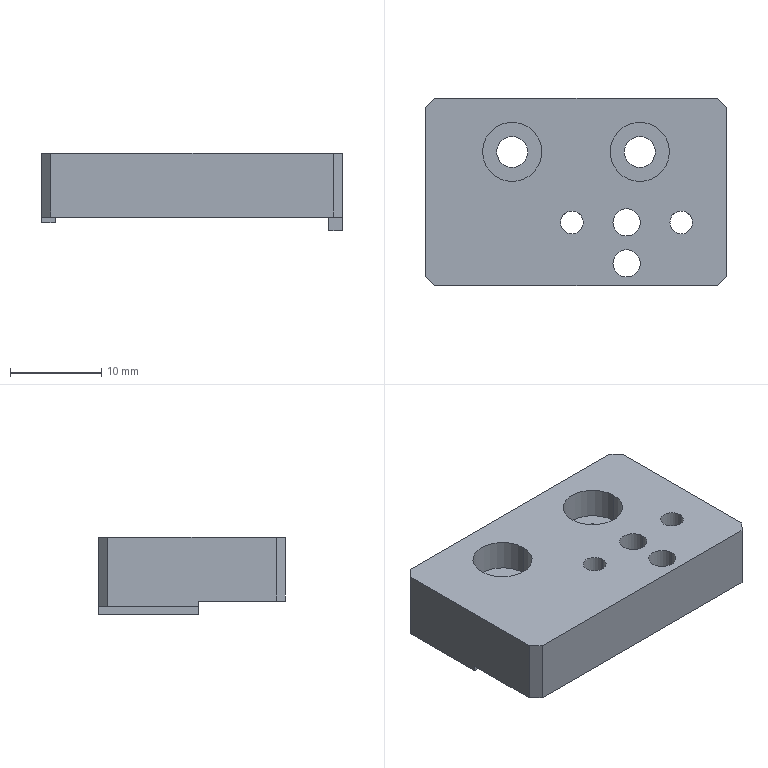Part | STEP file | 11-FG-E03511 | 1 solid | 34 faces | box 33 x 20.5 x 8.5 mm | volume 4296 mm3 | plane 18 | cylinder 16 | commonest cylinder face diameters 2.5 x4 3 x4 3.4 x4 6.5 x4
STEP:
#1=CARTESIAN_POINT('',(12.8,7.41,0.));
#2=VERTEX_POINT('',#1);
#3=CARTESIAN_POINT('',(10.3,7.41,0.));
#4=VERTEX_POINT('',#3);
#5=CARTESIAN_POINT('',(11.55,7.41,0.));
#6=DIRECTION('',(0.,0.,-1.));
#7=DIRECTION('',(-1.,0.,0.));
#8=AXIS2_PLACEMENT_3D('',#5,#6,#7);
#9=CIRCLE('',#8,1.25);
#10=EDGE_CURVE('',#2,#4,#9,.T.);
#11=ORIENTED_EDGE('',*,*,#10,.T.);
#12=CARTESIAN_POINT('',(10.3,7.41,7.));
#13=VERTEX_POINT('',#12);
#14=CARTESIAN_POINT('',(10.3,7.41,7.));
#15=DIRECTION('',(0.,0.,1.));
#16=VECTOR('',#15,1000.);
#17=LINE('',#14,#16);
#18=EDGE_CURVE('',#4,#13,#17,.T.);
#19=ORIENTED_EDGE('',*,*,#18,.T.);
#20=CARTESIAN_POINT('',(12.8,7.41,7.));
#21=VERTEX_POINT('',#20);
#22=CARTESIAN_POINT('',(11.55,7.41,7.));
#23=DIRECTION('',(0.,0.,1.));
#24=DIRECTION('',(1.,0.,0.));
#25=AXIS2_PLACEMENT_3D('',#22,#23,#24);
#26=CIRCLE('',#25,1.25);
#27=EDGE_CURVE('',#13,#21,#26,.T.);
#28=ORIENTED_EDGE('',*,*,#27,.T.);
#29=CARTESIAN_POINT('',(12.8,7.41,7.));
#30=DIRECTION('',(0.,0.,1.));
#31=VECTOR('',#30,1000.);
#32=LINE('',#29,#31);
#33=EDGE_CURVE('',#2,#21,#32,.T.);
#34=ORIENTED_EDGE('',*,*,#33,.F.);
#35=EDGE_LOOP('',(#11,#19,#28,#34));
#36=FACE_OUTER_BOUND('',#35,.T.);
#37=CARTESIAN_POINT('',(11.55,7.41,7.));
#38=DIRECTION('',(0.,0.,1.));
#39=DIRECTION('',(1.,0.,0.));
#40=AXIS2_PLACEMENT_3D('',#37,#38,#39);
#41=CYLINDRICAL_SURFACE('',#40,1.25);
#42=ADVANCED_FACE('',(#36),#41,.F.);
#43=CARTESIAN_POINT('',(0.7996,7.41,0.));
#44=VERTEX_POINT('',#43);
#45=CARTESIAN_POINT('',(-1.7,7.41,0.));
#46=VERTEX_POINT('',#45);
#47=CARTESIAN_POINT('',(-0.4504,7.41,0.));
#48=DIRECTION('',(0.,0.,-1.));
#49=DIRECTION('',(-1.,0.,0.));
#50=AXIS2_PLACEMENT_3D('',#47,#48,#49);
#51=CIRCLE('',#50,1.25);
#52=EDGE_CURVE('',#44,#46,#51,.T.);
#53=ORIENTED_EDGE('',*,*,#52,.T.);
#54=CARTESIAN_POINT('',(-1.7,7.41,7.));
#55=VERTEX_POINT('',#54);
#56=CARTESIAN_POINT('',(-1.7,7.41,7.));
#57=DIRECTION('',(0.,0.,1.));
#58=VECTOR('',#57,1000.);
#59=LINE('',#56,#58);
#60=EDGE_CURVE('',#46,#55,#59,.T.);
#61=ORIENTED_EDGE('',*,*,#60,.T.);
#62=CARTESIAN_POINT('',(0.7996,7.41,7.));
#63=VERTEX_POINT('',#62);
#64=CARTESIAN_POINT('',(-0.4504,7.41,7.));
#65=DIRECTION('',(0.,0.,1.));
#66=DIRECTION('',(1.,0.,0.));
#67=AXIS2_PLACEMENT_3D('',#64,#65,#66);
#68=CIRCLE('',#67,1.25);
#69=EDGE_CURVE('',#55,#63,#68,.T.);
#70=ORIENTED_EDGE('',*,*,#69,.T.);
#71=CARTESIAN_POINT('',(0.7996,7.41,7.));
#72=DIRECTION('',(0.,0.,1.));
#73=VECTOR('',#72,1000.);
#74=LINE('',#71,#73);
#75=EDGE_CURVE('',#44,#63,#74,.T.);
#76=ORIENTED_EDGE('',*,*,#75,.F.);
#77=EDGE_LOOP('',(#53,#61,#70,#76));
#78=FACE_OUTER_BOUND('',#77,.T.);
#79=CARTESIAN_POINT('',(-0.4504,7.41,7.));
#80=DIRECTION('',(0.,0.,1.));
#81=DIRECTION('',(1.,0.,0.));
#82=AXIS2_PLACEMENT_3D('',#79,#80,#81);
#83=CYLINDRICAL_SURFACE('',#82,1.25);
#84=ADVANCED_FACE('',(#78),#83,.F.);
#85=CARTESIAN_POINT('',(7.05,2.91,0.));
#86=VERTEX_POINT('',#85);
#87=CARTESIAN_POINT('',(4.05,2.91,0.));
#88=VERTEX_POINT('',#87);
#89=CARTESIAN_POINT('',(5.55,2.91,0.));
#90=DIRECTION('',(0.,0.,-1.));
#91=DIRECTION('',(-1.,0.,0.));
#92=AXIS2_PLACEMENT_3D('',#89,#90,#91);
#93=CIRCLE('',#92,1.5);
#94=EDGE_CURVE('',#86,#88,#93,.T.);
#95=ORIENTED_EDGE('',*,*,#94,.T.);
#96=CARTESIAN_POINT('',(4.05,2.91,7.));
#97=VERTEX_POINT('',#96);
#98=CARTESIAN_POINT('',(4.05,2.91,7.));
#99=DIRECTION('',(0.,0.,1.));
#100=VECTOR('',#99,1000.);
#101=LINE('',#98,#100);
#102=EDGE_CURVE('',#88,#97,#101,.T.);
#103=ORIENTED_EDGE('',*,*,#102,.T.);
#104=CARTESIAN_POINT('',(7.05,2.91,7.));
#105=VERTEX_POINT('',#104);
#106=CARTESIAN_POINT('',(5.55,2.91,7.));
#107=DIRECTION('',(0.,0.,1.));
#108=DIRECTION('',(1.,0.,0.));
#109=AXIS2_PLACEMENT_3D('',#106,#107,#108);
#110=CIRCLE('',#109,1.5);
#111=EDGE_CURVE('',#97,#105,#110,.T.);
#112=ORIENTED_EDGE('',*,*,#111,.T.);
#113=CARTESIAN_POINT('',(7.05,2.91,7.));
#114=DIRECTION('',(0.,0.,1.));
#115=VECTOR('',#114,1000.);
#116=LINE('',#113,#115);
#117=EDGE_CURVE('',#86,#105,#116,.T.);
#118=ORIENTED_EDGE('',*,*,#117,.F.);
#119=EDGE_LOOP('',(#95,#103,#112,#118));
#120=FACE_OUTER_BOUND('',#119,.T.);
#121=CARTESIAN_POINT('',(5.55,2.91,7.));
#122=DIRECTION('',(0.,0.,1.));
#123=DIRECTION('',(1.,0.,0.));
#124=AXIS2_PLACEMENT_3D('',#121,#122,#123);
#125=CYLINDRICAL_SURFACE('',#124,1.5);
#126=ADVANCED_FACE('',(#120),#125,.F.);
#127=CARTESIAN_POINT('',(7.05,7.41,0.));
#128=VERTEX_POINT('',#127);
#129=CARTESIAN_POINT('',(4.05,7.41,0.));
#130=VERTEX_POINT('',#129);
#131=CARTESIAN_POINT('',(5.55,7.41,0.));
#132=DIRECTION('',(0.,0.,-1.));
#133=DIRECTION('',(-1.,0.,0.));
#134=AXIS2_PLACEMENT_3D('',#131,#132,#133);
#135=CIRCLE('',#134,1.5);
#136=EDGE_CURVE('',#128,#130,#135,.T.);
#137=ORIENTED_EDGE('',*,*,#136,.T.);
#138=CARTESIAN_POINT('',(4.05,7.41,7.));
#139=VERTEX_POINT('',#138);
#140=CARTESIAN_POINT('',(4.05,7.41,7.));
#141=DIRECTION('',(0.,0.,1.));
#142=VECTOR('',#141,1000.);
#143=LINE('',#140,#142);
#144=EDGE_CURVE('',#130,#139,#143,.T.);
#145=ORIENTED_EDGE('',*,*,#144,.T.);
#146=CARTESIAN_POINT('',(7.05,7.41,7.));
#147=VERTEX_POINT('',#146);
#148=CARTESIAN_POINT('',(5.55,7.41,7.));
#149=DIRECTION('',(0.,0.,1.));
#150=DIRECTION('',(1.,0.,0.));
#151=AXIS2_PLACEMENT_3D('',#148,#149,#150);
#152=CIRCLE('',#151,1.5);
#153=EDGE_CURVE('',#139,#147,#152,.T.);
#154=ORIENTED_EDGE('',*,*,#153,.T.);
#155=CARTESIAN_POINT('',(7.05,7.41,7.));
#156=DIRECTION('',(0.,0.,1.));
#157=VECTOR('',#156,1000.);
#158=LINE('',#155,#157);
#159=EDGE_CURVE('',#128,#147,#158,.T.);
#160=ORIENTED_EDGE('',*,*,#159,.F.);
#161=EDGE_LOOP('',(#137,#145,#154,#160));
#162=FACE_OUTER_BOUND('',#161,.T.);
#163=CARTESIAN_POINT('',(5.55,7.41,7.));
#164=DIRECTION('',(0.,0.,1.));
#165=DIRECTION('',(1.,0.,0.));
#166=AXIS2_PLACEMENT_3D('',#163,#164,#165);
#167=CYLINDRICAL_SURFACE('',#166,1.5);
#168=ADVANCED_FACE('',(#162),#167,.F.);
#169=CARTESIAN_POINT('',(-10.25,15.147,3.6));
#170=VERTEX_POINT('',#169);
#171=CARTESIAN_POINT('',(-3.75,15.147,3.6));
#172=VERTEX_POINT('',#171);
#173=CARTESIAN_POINT('',(-7.,15.147,3.6));
#174=DIRECTION('',(0.,0.,1.));
#175=DIRECTION('',(1.,0.,0.));
#176=AXIS2_PLACEMENT_3D('',#173,#174,#175);
#177=CIRCLE('',#176,3.25);
#178=EDGE_CURVE('',#170,#172,#177,.T.);
#179=ORIENTED_EDGE('',*,*,#178,.F.);
#180=CARTESIAN_POINT('',(-10.25,15.147,7.));
#181=VERTEX_POINT('',#180);
#182=CARTESIAN_POINT('',(-10.25,15.147,7.));
#183=DIRECTION('',(0.,0.,1.));
#184=VECTOR('',#183,1000.);
#185=LINE('',#182,#184);
#186=EDGE_CURVE('',#170,#181,#185,.T.);
#187=ORIENTED_EDGE('',*,*,#186,.T.);
#188=CARTESIAN_POINT('',(-3.75,15.147,7.));
#189=VERTEX_POINT('',#188);
#190=CARTESIAN_POINT('',(-7.,15.147,7.));
#191=DIRECTION('',(0.,0.,1.));
#192=DIRECTION('',(1.,0.,0.));
#193=AXIS2_PLACEMENT_3D('',#190,#191,#192);
#194=CIRCLE('',#193,3.25);
#195=EDGE_CURVE('',#181,#189,#194,.T.);
#196=ORIENTED_EDGE('',*,*,#195,.T.);
#197=CARTESIAN_POINT('',(-3.75,15.147,7.));
#198=DIRECTION('',(0.,0.,1.));
#199=VECTOR('',#198,1000.);
#200=LINE('',#197,#199);
#201=EDGE_CURVE('',#172,#189,#200,.T.);
#202=ORIENTED_EDGE('',*,*,#201,.F.);
#203=EDGE_LOOP('',(#179,#187,#196,#202));
#204=FACE_OUTER_BOUND('',#203,.T.);
#205=CARTESIAN_POINT('',(-7.,15.147,7.));
#206=DIRECTION('',(0.,0.,1.));
#207=DIRECTION('',(1.,0.,0.));
#208=AXIS2_PLACEMENT_3D('',#205,#206,#207);
#209=CYLINDRICAL_SURFACE('',#208,3.25);
#210=ADVANCED_FACE('',(#204),#209,.F.);
#211=CARTESIAN_POINT('',(-8.7,15.147,0.));
#212=VERTEX_POINT('',#211);
#213=CARTESIAN_POINT('',(-5.3,15.147,0.));
#214=VERTEX_POINT('',#213);
#215=CARTESIAN_POINT('',(-7.,15.147,0.));
#216=DIRECTION('',(0.,0.,1.));
#217=DIRECTION('',(1.,0.,0.));
#218=AXIS2_PLACEMENT_3D('',#215,#216,#217);
#219=CIRCLE('',#218,1.7);
#220=EDGE_CURVE('',#212,#214,#219,.T.);
#221=ORIENTED_EDGE('',*,*,#220,.F.);
#222=CARTESIAN_POINT('',(-8.7,15.147,3.6));
#223=VERTEX_POINT('',#222);
#224=CARTESIAN_POINT('',(-8.7,15.147,7.));
#225=DIRECTION('',(0.,0.,1.));
#226=VECTOR('',#225,1000.);
#227=LINE('',#224,#226);
#228=EDGE_CURVE('',#212,#223,#227,.T.);
#229=ORIENTED_EDGE('',*,*,#228,.T.);
#230=CARTESIAN_POINT('',(-5.3,15.147,3.6));
#231=VERTEX_POINT('',#230);
#232=CARTESIAN_POINT('',(-7.,15.147,3.6));
#233=DIRECTION('',(0.,0.,1.));
#234=DIRECTION('',(1.,0.,0.));
#235=AXIS2_PLACEMENT_3D('',#232,#233,#234);
#236=CIRCLE('',#235,1.7);
#237=EDGE_CURVE('',#223,#231,#236,.T.);
#238=ORIENTED_EDGE('',*,*,#237,.T.);
#239=CARTESIAN_POINT('',(-5.3,15.147,7.));
#240=DIRECTION('',(0.,0.,1.));
#241=VECTOR('',#240,1000.);
#242=LINE('',#239,#241);
#243=EDGE_CURVE('',#214,#231,#242,.T.);
#244=ORIENTED_EDGE('',*,*,#243,.F.);
#245=EDGE_LOOP('',(#221,#229,#238,#244));
#246=FACE_OUTER_BOUND('',#245,.T.);
#247=CARTESIAN_POINT('',(-7.,15.147,7.));
#248=DIRECTION('',(0.,0.,1.));
#249=DIRECTION('',(1.,0.,0.));
#250=AXIS2_PLACEMENT_3D('',#247,#248,#249);
#251=CYLINDRICAL_SURFACE('',#250,1.7);
#252=ADVANCED_FACE('',(#246),#251,.F.);
#253=CARTESIAN_POINT('',(3.75,15.147,3.6));
#254=VERTEX_POINT('',#253);
#255=CARTESIAN_POINT('',(10.25,15.147,3.6));
#256=VERTEX_POINT('',#255);
#257=CARTESIAN_POINT('',(7.,15.147,3.6));
#258=DIRECTION('',(0.,0.,1.));
#259=DIRECTION('',(1.,0.,0.));
#260=AXIS2_PLACEMENT_3D('',#257,#258,#259);
#261=CIRCLE('',#260,3.25);
#262=EDGE_CURVE('',#254,#256,#261,.T.);
#263=ORIENTED_EDGE('',*,*,#262,.F.);
#264=CARTESIAN_POINT('',(3.75,15.147,7.));
#265=VERTEX_POINT('',#264);
#266=CARTESIAN_POINT('',(3.75,15.147,7.));
#267=DIRECTION('',(0.,0.,1.));
#268=VECTOR('',#267,1000.);
#269=LINE('',#266,#268);
#270=EDGE_CURVE('',#254,#265,#269,.T.);
#271=ORIENTED_EDGE('',*,*,#270,.T.);
#272=CARTESIAN_POINT('',(10.25,15.147,7.));
#273=VERTEX_POINT('',#272);
#274=CARTESIAN_POINT('',(7.,15.147,7.));
#275=DIRECTION('',(0.,0.,1.));
#276=DIRECTION('',(1.,0.,0.));
#277=AXIS2_PLACEMENT_3D('',#274,#275,#276);
#278=CIRCLE('',#277,3.25);
#279=EDGE_CURVE('',#265,#273,#278,.T.);
#280=ORIENTED_EDGE('',*,*,#279,.T.);
#281=CARTESIAN_POINT('',(10.25,15.147,7.));
#282=DIRECTION('',(0.,0.,1.));
#283=VECTOR('',#282,1000.);
#284=LINE('',#281,#283);
#285=EDGE_CURVE('',#256,#273,#284,.T.);
#286=ORIENTED_EDGE('',*,*,#285,.F.);
#287=EDGE_LOOP('',(#263,#271,#280,#286));
#288=FACE_OUTER_BOUND('',#287,.T.);
#289=CARTESIAN_POINT('',(7.,15.147,7.));
#290=DIRECTION('',(0.,0.,1.));
#291=DIRECTION('',(1.,0.,0.));
#292=AXIS2_PLACEMENT_3D('',#289,#290,#291);
#293=CYLINDRICAL_SURFACE('',#292,3.25);
#294=ADVANCED_FACE('',(#288),#293,.F.);
#295=CARTESIAN_POINT('',(5.3,15.147,0.));
#296=VERTEX_POINT('',#295);
#297=CARTESIAN_POINT('',(8.7,15.147,0.));
#298=VERTEX_POINT('',#297);
#299=CARTESIAN_POINT('',(7.,15.147,0.));
#300=DIRECTION('',(0.,0.,1.));
#301=DIRECTION('',(1.,0.,0.));
#302=AXIS2_PLACEMENT_3D('',#299,#300,#301);
#303=CIRCLE('',#302,1.7);
#304=EDGE_CURVE('',#296,#298,#303,.T.);
#305=ORIENTED_EDGE('',*,*,#304,.F.);
#306=CARTESIAN_POINT('',(5.3,15.147,3.6));
#307=VERTEX_POINT('',#306);
#308=CARTESIAN_POINT('',(5.3,15.147,7.));
#309=DIRECTION('',(0.,0.,1.));
#310=VECTOR('',#309,1000.);
#311=LINE('',#308,#310);
#312=EDGE_CURVE('',#296,#307,#311,.T.);
#313=ORIENTED_EDGE('',*,*,#312,.T.);
#314=CARTESIAN_POINT('',(8.7,15.147,3.6));
#315=VERTEX_POINT('',#314);
#316=CARTESIAN_POINT('',(7.,15.147,3.6));
#317=DIRECTION('',(0.,0.,1.));
#318=DIRECTION('',(1.,0.,0.));
#319=AXIS2_PLACEMENT_3D('',#316,#317,#318);
#320=CIRCLE('',#319,1.7);
#321=EDGE_CURVE('',#307,#315,#320,.T.);
#322=ORIENTED_EDGE('',*,*,#321,.T.);
#323=CARTESIAN_POINT('',(8.7,15.147,7.));
#324=DIRECTION('',(0.,0.,1.));
#325=VECTOR('',#324,1000.);
#326=LINE('',#323,#325);
#327=EDGE_CURVE('',#298,#315,#326,.T.);
#328=ORIENTED_EDGE('',*,*,#327,.F.);
#329=EDGE_LOOP('',(#305,#313,#322,#328));
#330=FACE_OUTER_BOUND('',#329,.T.);
#331=CARTESIAN_POINT('',(7.,15.147,7.));
#332=DIRECTION('',(0.,0.,1.));
#333=DIRECTION('',(1.,0.,0.));
#334=AXIS2_PLACEMENT_3D('',#331,#332,#333);
#335=CYLINDRICAL_SURFACE('',#334,1.7);
#336=ADVANCED_FACE('',(#330),#335,.F.);
#337=ORIENTED_EDGE('',*,*,#10,.F.);
#338=CARTESIAN_POINT('',(11.55,7.41,0.));
#339=DIRECTION('',(0.,0.,-1.));
#340=DIRECTION('',(-1.,0.,0.));
#341=AXIS2_PLACEMENT_3D('',#338,#339,#340);
#342=CIRCLE('',#341,1.25);
#343=EDGE_CURVE('',#4,#2,#342,.T.);
#344=ORIENTED_EDGE('',*,*,#343,.F.);
#345=EDGE_LOOP('',(#337,#344));
#346=FACE_BOUND('',#345,.T.);
#347=ORIENTED_EDGE('',*,*,#52,.F.);
#348=CARTESIAN_POINT('',(-0.4504,7.41,0.));
#349=DIRECTION('',(0.,0.,-1.));
#350=DIRECTION('',(-1.,0.,0.));
#351=AXIS2_PLACEMENT_3D('',#348,#349,#350);
#352=CIRCLE('',#351,1.25);
#353=EDGE_CURVE('',#46,#44,#352,.T.);
#354=ORIENTED_EDGE('',*,*,#353,.F.);
#355=EDGE_LOOP('',(#347,#354));
#356=FACE_BOUND('',#355,.T.);
#357=ORIENTED_EDGE('',*,*,#94,.F.);
#358=CARTESIAN_POINT('',(5.55,2.91,0.));
#359=DIRECTION('',(0.,0.,-1.));
#360=DIRECTION('',(-1.,0.,0.));
#361=AXIS2_PLACEMENT_3D('',#358,#359,#360);
#362=CIRCLE('',#361,1.5);
#363=EDGE_CURVE('',#88,#86,#362,.T.);
#364=ORIENTED_EDGE('',*,*,#363,.F.);
#365=EDGE_LOOP('',(#357,#364));
#366=FACE_BOUND('',#365,.T.);
#367=ORIENTED_EDGE('',*,*,#136,.F.);
#368=CARTESIAN_POINT('',(5.55,7.41,0.));
#369=DIRECTION('',(0.,0.,-1.));
#370=DIRECTION('',(-1.,0.,0.));
#371=AXIS2_PLACEMENT_3D('',#368,#369,#370);
#372=CIRCLE('',#371,1.5);
#373=EDGE_CURVE('',#130,#128,#372,.T.);
#374=ORIENTED_EDGE('',*,*,#373,.F.);
#375=EDGE_LOOP('',(#367,#374));
#376=FACE_BOUND('',#375,.T.);
#377=CARTESIAN_POINT('',(-15.5,0.5,0.));
#378=VERTEX_POINT('',#377);
#379=CARTESIAN_POINT('',(15.5,0.5,0.));
#380=VERTEX_POINT('',#379);
#381=CARTESIAN_POINT('',(0.,0.5,0.));
#382=DIRECTION('',(1.,0.,0.));
#383=VECTOR('',#382,1000.);
#384=LINE('',#381,#383);
#385=EDGE_CURVE('',#378,#380,#384,.T.);
#386=ORIENTED_EDGE('',*,*,#385,.F.);
#387=CARTESIAN_POINT('',(-16.5,1.5,0.));
#388=VERTEX_POINT('',#387);
#389=CARTESIAN_POINT('',(-7.5,-7.5,0.));
#390=DIRECTION('',(-0.7071,0.7071,0.));
#391=VECTOR('',#390,1000.);
#392=LINE('',#389,#391);
#393=EDGE_CURVE('',#378,#388,#392,.T.);
#394=ORIENTED_EDGE('',*,*,#393,.T.);
#395=CARTESIAN_POINT('',(-16.5,10.,0.));
#396=VERTEX_POINT('',#395);
#397=CARTESIAN_POINT('',(-16.5,0.,0.));
#398=DIRECTION('',(0.,-1.,0.));
#399=VECTOR('',#398,1000.);
#400=LINE('',#397,#399);
#401=EDGE_CURVE('',#396,#388,#400,.T.);
#402=ORIENTED_EDGE('',*,*,#401,.F.);
#403=CARTESIAN_POINT('',(-15.,10.,0.));
#404=VERTEX_POINT('',#403);
#405=CARTESIAN_POINT('',(-23.4,10.,0.));
#406=DIRECTION('',(-1.,0.,0.));
#407=VECTOR('',#406,1000.);
#408=LINE('',#405,#407);
#409=EDGE_CURVE('',#404,#396,#408,.T.);
#410=ORIENTED_EDGE('',*,*,#409,.F.);
#411=CARTESIAN_POINT('',(-15.,21.,0.));
#412=VERTEX_POINT('',#411);
#413=CARTESIAN_POINT('',(-15.,21.,0.));
#414=DIRECTION('',(0.,-1.,0.));
#415=VECTOR('',#414,1000.);
#416=LINE('',#413,#415);
#417=EDGE_CURVE('',#412,#404,#416,.T.);
#418=ORIENTED_EDGE('',*,*,#417,.F.);
#419=CARTESIAN_POINT('',(15.,21.,0.));
#420=VERTEX_POINT('',#419);
#421=CARTESIAN_POINT('',(-27.5,21.,0.));
#422=DIRECTION('',(-1.,0.,0.));
#423=VECTOR('',#422,1000.);
#424=LINE('',#421,#423);
#425=EDGE_CURVE('',#420,#412,#424,.T.);
#426=ORIENTED_EDGE('',*,*,#425,.F.);
#427=CARTESIAN_POINT('',(15.,10.,0.));
#428=VERTEX_POINT('',#427);
#429=CARTESIAN_POINT('',(15.,10.,0.));
#430=DIRECTION('',(0.,1.,0.));
#431=VECTOR('',#430,1000.);
#432=LINE('',#429,#431);
#433=EDGE_CURVE('',#428,#420,#432,.T.);
#434=ORIENTED_EDGE('',*,*,#433,.F.);
#435=CARTESIAN_POINT('',(16.5,10.,0.));
#436=VERTEX_POINT('',#435);
#437=CARTESIAN_POINT('',(21.6,10.,0.));
#438=DIRECTION('',(-1.,0.,0.));
#439=VECTOR('',#438,1000.);
#440=LINE('',#437,#439);
#441=EDGE_CURVE('',#436,#428,#440,.T.);
#442=ORIENTED_EDGE('',*,*,#441,.F.);
#443=CARTESIAN_POINT('',(16.5,1.5,0.));
#444=VERTEX_POINT('',#443);
#445=CARTESIAN_POINT('',(16.5,0.,0.));
#446=DIRECTION('',(0.,1.,0.));
#447=VECTOR('',#446,1000.);
#448=LINE('',#445,#447);
#449=EDGE_CURVE('',#444,#436,#448,.T.);
#450=ORIENTED_EDGE('',*,*,#449,.F.);
#451=CARTESIAN_POINT('',(7.5,-7.5,0.));
#452=DIRECTION('',(-0.7071,-0.7071,0.));
#453=VECTOR('',#452,1000.);
#454=LINE('',#451,#453);
#455=EDGE_CURVE('',#444,#380,#454,.T.);
#456=ORIENTED_EDGE('',*,*,#455,.T.);
#457=EDGE_LOOP('',(#386,#394,#402,#410,#418,#426,#434,#442,#450,#456));
#458=FACE_OUTER_BOUND('',#457,.T.);
#459=CARTESIAN_POINT('',(-7.,15.147,0.));
#460=DIRECTION('',(0.,0.,1.));
#461=DIRECTION('',(1.,0.,0.));
#462=AXIS2_PLACEMENT_3D('',#459,#460,#461);
#463=CIRCLE('',#462,1.7);
#464=EDGE_CURVE('',#214,#212,#463,.T.);
#465=ORIENTED_EDGE('',*,*,#464,.T.);
#466=ORIENTED_EDGE('',*,*,#220,.T.);
#467=EDGE_LOOP('',(#465,#466));
#468=FACE_BOUND('',#467,.T.);
#469=CARTESIAN_POINT('',(7.,15.147,0.));
#470=DIRECTION('',(0.,0.,1.));
#471=DIRECTION('',(1.,0.,0.));
#472=AXIS2_PLACEMENT_3D('',#469,#470,#471);
#473=CIRCLE('',#472,1.7);
#474=EDGE_CURVE('',#298,#296,#473,.T.);
#475=ORIENTED_EDGE('',*,*,#474,.T.);
#476=ORIENTED_EDGE('',*,*,#304,.T.);
#477=EDGE_LOOP('',(#475,#476));
#478=FACE_BOUND('',#477,.T.);
#479=CARTESIAN_POINT('',(0.,0.,0.));
#480=DIRECTION('',(0.,0.,-1.));
#481=DIRECTION('',(-1.,0.,0.));
#482=AXIS2_PLACEMENT_3D('',#479,#480,#481);
#483=PLANE('',#482);
#484=ADVANCED_FACE('',(#346,#356,#366,#376,#458,#468,#478),#483,.T.);
#485=CARTESIAN_POINT('',(15.5,21.,7.));
#486=VERTEX_POINT('',#485);
#487=CARTESIAN_POINT('',(-15.5,21.,7.));
#488=VERTEX_POINT('',#487);
#489=CARTESIAN_POINT('',(-27.5,21.,7.));
#490=DIRECTION('',(-1.,0.,0.));
#491=VECTOR('',#490,1000.);
#492=LINE('',#489,#491);
#493=EDGE_CURVE('',#486,#488,#492,.T.);
#494=ORIENTED_EDGE('',*,*,#493,.F.);
#495=CARTESIAN_POINT('',(15.5,21.,-1.5));
#496=VERTEX_POINT('',#495);
#497=CARTESIAN_POINT('',(15.5,21.,7.));
#498=DIRECTION('',(0.,0.,-1.));
#499=VECTOR('',#498,1000.);
#500=LINE('',#497,#499);
#501=EDGE_CURVE('',#486,#496,#500,.T.);
#502=ORIENTED_EDGE('',*,*,#501,.T.);
#503=CARTESIAN_POINT('',(15.,21.,-1.5));
#504=VERTEX_POINT('',#503);
#505=CARTESIAN_POINT('',(-16.5,21.,-1.5));
#506=DIRECTION('',(1.,0.,0.));
#507=VECTOR('',#506,1000.);
#508=LINE('',#505,#507);
#509=EDGE_CURVE('',#504,#496,#508,.T.);
#510=ORIENTED_EDGE('',*,*,#509,.F.);
#511=CARTESIAN_POINT('',(15.,21.,-2.));
#512=DIRECTION('',(0.,0.,1.));
#513=VECTOR('',#512,1000.);
#514=LINE('',#511,#513);
#515=EDGE_CURVE('',#504,#420,#514,.T.);
#516=ORIENTED_EDGE('',*,*,#515,.T.);
#517=ORIENTED_EDGE('',*,*,#425,.T.);
#518=CARTESIAN_POINT('',(-15.,21.,-0.6));
#519=VERTEX_POINT('',#518);
#520=CARTESIAN_POINT('',(-15.,21.,-2.));
#521=DIRECTION('',(0.,0.,1.));
#522=VECTOR('',#521,1000.);
#523=LINE('',#520,#522);
#524=EDGE_CURVE('',#519,#412,#523,.T.);
#525=ORIENTED_EDGE('',*,*,#524,.F.);
#526=CARTESIAN_POINT('',(-15.5,21.,-0.6));
#527=VERTEX_POINT('',#526);
#528=CARTESIAN_POINT('',(-15.,21.,-0.6));
#529=DIRECTION('',(1.,0.,0.));
#530=VECTOR('',#529,1000.);
#531=LINE('',#528,#530);
#532=EDGE_CURVE('',#527,#519,#531,.T.);
#533=ORIENTED_EDGE('',*,*,#532,.F.);
#534=CARTESIAN_POINT('',(-15.5,21.,7.));
#535=DIRECTION('',(0.,0.,1.));
#536=VECTOR('',#535,1000.);
#537=LINE('',#534,#536);
#538=EDGE_CURVE('',#527,#488,#537,.T.);
#539=ORIENTED_EDGE('',*,*,#538,.T.);
#540=EDGE_LOOP('',(#494,#502,#510,#516,#517,#525,#533,#539));
#541=FACE_OUTER_BOUND('',#540,.T.);
#542=CARTESIAN_POINT('',(-27.5,21.,7.));
#543=DIRECTION('',(0.,-1.,0.));
#544=DIRECTION('',(0.,0.,-1.));
#545=AXIS2_PLACEMENT_3D('',#542,#543,#544);
#546=PLANE('',#545);
#547=ADVANCED_FACE('',(#541),#546,.F.);
#548=CARTESIAN_POINT('',(11.55,7.41,7.));
#549=DIRECTION('',(0.,0.,1.));
#550=DIRECTION('',(1.,0.,0.));
#551=AXIS2_PLACEMENT_3D('',#548,#549,#550);
#552=CIRCLE('',#551,1.25);
#553=EDGE_CURVE('',#21,#13,#552,.T.);
#554=ORIENTED_EDGE('',*,*,#553,.F.);
#555=ORIENTED_EDGE('',*,*,#27,.F.);
#556=EDGE_LOOP('',(#554,#555));
#557=FACE_BOUND('',#556,.T.);
#558=CARTESIAN_POINT('',(-0.4504,7.41,7.));
#559=DIRECTION('',(0.,0.,1.));
#560=DIRECTION('',(1.,0.,0.));
#561=AXIS2_PLACEMENT_3D('',#558,#559,#560);
#562=CIRCLE('',#561,1.25);
#563=EDGE_CURVE('',#63,#55,#562,.T.);
#564=ORIENTED_EDGE('',*,*,#563,.F.);
#565=ORIENTED_EDGE('',*,*,#69,.F.);
#566=EDGE_LOOP('',(#564,#565));
#567=FACE_BOUND('',#566,.T.);
#568=CARTESIAN_POINT('',(5.55,2.91,7.));
#569=DIRECTION('',(0.,0.,1.));
#570=DIRECTION('',(1.,0.,0.));
#571=AXIS2_PLACEMENT_3D('',#568,#569,#570);
#572=CIRCLE('',#571,1.5);
#573=EDGE_CURVE('',#105,#97,#572,.T.);
#574=ORIENTED_EDGE('',*,*,#573,.F.);
#575=ORIENTED_EDGE('',*,*,#111,.F.);
#576=EDGE_LOOP('',(#574,#575));
#577=FACE_BOUND('',#576,.T.);
#578=CARTESIAN_POINT('',(5.55,7.41,7.));
#579=DIRECTION('',(0.,0.,1.));
#580=DIRECTION('',(1.,0.,0.));
#581=AXIS2_PLACEMENT_3D('',#578,#579,#580);
#582=CIRCLE('',#581,1.5);
#583=EDGE_CURVE('',#147,#139,#582,.T.);
#584=ORIENTED_EDGE('',*,*,#583,.F.);
#585=ORIENTED_EDGE('',*,*,#153,.F.);
#586=EDGE_LOOP('',(#584,#585));
#587=FACE_BOUND('',#586,.T.);
#588=CARTESIAN_POINT('',(-7.,15.147,7.));
#589=DIRECTION('',(0.,0.,1.));
#590=DIRECTION('',(1.,0.,0.));
#591=AXIS2_PLACEMENT_3D('',#588,#589,#590);
#592=CIRCLE('',#591,3.25);
#593=EDGE_CURVE('',#189,#181,#592,.T.);
#594=ORIENTED_EDGE('',*,*,#593,.F.);
#595=ORIENTED_EDGE('',*,*,#195,.F.);
#596=EDGE_LOOP('',(#594,#595));
#597=FACE_BOUND('',#596,.T.);
#598=CARTESIAN_POINT('',(7.,15.147,7.));
#599=DIRECTION('',(0.,0.,1.));
#600=DIRECTION('',(1.,0.,0.));
#601=AXIS2_PLACEMENT_3D('',#598,#599,#600);
#602=CIRCLE('',#601,3.25);
#603=EDGE_CURVE('',#273,#265,#602,.T.);
#604=ORIENTED_EDGE('',*,*,#603,.F.);
#605=ORIENTED_EDGE('',*,*,#279,.F.);
#606=EDGE_LOOP('',(#604,#605));
#607=FACE_BOUND('',#606,.T.);
#608=CARTESIAN_POINT('',(16.5,20.,7.));
#609=VERTEX_POINT('',#608);
#610=CARTESIAN_POINT('',(16.5,1.5,7.));
#611=VERTEX_POINT('',#610);
#612=CARTESIAN_POINT('',(16.5,21.,7.));
#613=DIRECTION('',(0.,-1.,0.));
#614=VECTOR('',#613,1000.);
#615=LINE('',#612,#614);
#616=EDGE_CURVE('',#609,#611,#615,.T.);
#617=ORIENTED_EDGE('',*,*,#616,.F.);
#618=CARTESIAN_POINT('',(16.5,20.,7.));
#619=DIRECTION('',(-0.7071,0.7071,0.));
#620=VECTOR('',#619,1000.);
#621=LINE('',#618,#620);
#622=EDGE_CURVE('',#609,#486,#621,.T.);
#623=ORIENTED_EDGE('',*,*,#622,.T.);
#624=ORIENTED_EDGE('',*,*,#493,.T.);
#625=CARTESIAN_POINT('',(-16.5,20.,7.));
#626=VERTEX_POINT('',#625);
#627=CARTESIAN_POINT('',(-16.5,20.,7.));
#628=DIRECTION('',(-0.7071,-0.7071,0.));
#629=VECTOR('',#628,1000.);
#630=LINE('',#627,#629);
#631=EDGE_CURVE('',#488,#626,#630,.T.);
#632=ORIENTED_EDGE('',*,*,#631,.T.);
#633=CARTESIAN_POINT('',(-16.5,1.5,7.));
#634=VERTEX_POINT('',#633);
#635=CARTESIAN_POINT('',(-16.5,-20.,7.));
#636=DIRECTION('',(0.,1.,0.));
#637=VECTOR('',#636,1000.);
#638=LINE('',#635,#637);
#639=EDGE_CURVE('',#634,#626,#638,.T.);
#640=ORIENTED_EDGE('',*,*,#639,.F.);
#641=CARTESIAN_POINT('',(-15.5,0.5,7.));
#642=VERTEX_POINT('',#641);
#643=CARTESIAN_POINT('',(-15.5,0.5,7.));
#644=DIRECTION('',(0.7071,-0.7071,0.));
#645=VECTOR('',#644,1000.);
#646=LINE('',#643,#645);
#647=EDGE_CURVE('',#634,#642,#646,.T.);
#648=ORIENTED_EDGE('',*,*,#647,.T.);
#649=CARTESIAN_POINT('',(15.5,0.5,7.));
#650=VERTEX_POINT('',#649);
#651=CARTESIAN_POINT('',(27.5,0.5,7.));
#652=DIRECTION('',(-1.,0.,0.));
#653=VECTOR('',#652,1000.);
#654=LINE('',#651,#653);
#655=EDGE_CURVE('',#650,#642,#654,.T.);
#656=ORIENTED_EDGE('',*,*,#655,.F.);
#657=CARTESIAN_POINT('',(15.5,0.5,7.));
#658=DIRECTION('',(0.7071,0.7071,0.));
#659=VECTOR('',#658,1000.);
#660=LINE('',#657,#659);
#661=EDGE_CURVE('',#650,#611,#660,.T.);
#662=ORIENTED_EDGE('',*,*,#661,.T.);
#663=EDGE_LOOP('',(#617,#623,#624,#632,#640,#648,#656,#662));
#664=FACE_OUTER_BOUND('',#663,.T.);
#665=CARTESIAN_POINT('',(0.,0.,7.));
#666=DIRECTION('',(0.,0.,-1.));
#667=DIRECTION('',(-1.,0.,0.));
#668=AXIS2_PLACEMENT_3D('',#665,#666,#667);
#669=PLANE('',#668);
#670=ADVANCED_FACE('',(#557,#567,#577,#587,#597,#607,#664),#669,.F.);
#671=ORIENTED_EDGE('',*,*,#655,.T.);
#672=CARTESIAN_POINT('',(-15.5,0.5,-3.));
#673=DIRECTION('',(0.,0.,-1.));
#674=VECTOR('',#673,1000.);
#675=LINE('',#672,#674);
#676=EDGE_CURVE('',#642,#378,#675,.T.);
#677=ORIENTED_EDGE('',*,*,#676,.T.);
#678=ORIENTED_EDGE('',*,*,#385,.T.);
#679=CARTESIAN_POINT('',(15.5,0.5,-3.));
#680=DIRECTION('',(0.,0.,1.));
#681=VECTOR('',#680,1000.);
#682=LINE('',#679,#681);
#683=EDGE_CURVE('',#380,#650,#682,.T.);
#684=ORIENTED_EDGE('',*,*,#683,.T.);
#685=EDGE_LOOP('',(#671,#677,#678,#684));
#686=FACE_OUTER_BOUND('',#685,.T.);
#687=CARTESIAN_POINT('',(27.5,0.5,-3.));
#688=DIRECTION('',(0.,1.,0.));
#689=DIRECTION('',(-1.,0.,0.));
#690=AXIS2_PLACEMENT_3D('',#687,#688,#689);
#691=PLANE('',#690);
#692=ADVANCED_FACE('',(#686),#691,.F.);
#693=ORIENTED_EDGE('',*,*,#312,.F.);
#694=ORIENTED_EDGE('',*,*,#474,.F.);
#695=ORIENTED_EDGE('',*,*,#327,.T.);
#696=CARTESIAN_POINT('',(7.,15.147,3.6));
#697=DIRECTION('',(0.,0.,1.));
#698=DIRECTION('',(1.,0.,0.));
#699=AXIS2_PLACEMENT_3D('',#696,#697,#698);
#700=CIRCLE('',#699,1.7);
#701=EDGE_CURVE('',#315,#307,#700,.T.);
#702=ORIENTED_EDGE('',*,*,#701,.T.);
#703=EDGE_LOOP('',(#693,#694,#695,#702));
#704=FACE_OUTER_BOUND('',#703,.T.);
#705=CARTESIAN_POINT('',(7.,15.147,7.));
#706=DIRECTION('',(0.,0.,1.));
#707=DIRECTION('',(1.,0.,0.));
#708=AXIS2_PLACEMENT_3D('',#705,#706,#707);
#709=CYLINDRICAL_SURFACE('',#708,1.7);
#710=ADVANCED_FACE('',(#704),#709,.F.);
#711=ORIENTED_EDGE('',*,*,#701,.F.);
#712=ORIENTED_EDGE('',*,*,#321,.F.);
#713=EDGE_LOOP('',(#711,#712));
#714=FACE_BOUND('',#713,.T.);
#715=CARTESIAN_POINT('',(7.,15.147,3.6));
#716=DIRECTION('',(0.,0.,1.));
#717=DIRECTION('',(1.,0.,0.));
#718=AXIS2_PLACEMENT_3D('',#715,#716,#717);
#719=CIRCLE('',#718,3.25);
#720=EDGE_CURVE('',#256,#254,#719,.T.);
#721=ORIENTED_EDGE('',*,*,#720,.T.);
#722=ORIENTED_EDGE('',*,*,#262,.T.);
#723=EDGE_LOOP('',(#721,#722));
#724=FACE_OUTER_BOUND('',#723,.T.);
#725=CARTESIAN_POINT('',(8.7,15.147,3.6));
#726=DIRECTION('',(0.,0.,-1.));
#727=DIRECTION('',(-1.,0.,0.));
#728=AXIS2_PLACEMENT_3D('',#725,#726,#727);
#729=PLANE('',#728);
#730=ADVANCED_FACE('',(#714,#724),#729,.F.);
#731=ORIENTED_EDGE('',*,*,#270,.F.);
#732=ORIENTED_EDGE('',*,*,#720,.F.);
#733=ORIENTED_EDGE('',*,*,#285,.T.);
#734=ORIENTED_EDGE('',*,*,#603,.T.);
#735=EDGE_LOOP('',(#731,#732,#733,#734));
#736=FACE_OUTER_BOUND('',#735,.T.);
#737=CARTESIAN_POINT('',(7.,15.147,7.));
#738=DIRECTION('',(0.,0.,1.));
#739=DIRECTION('',(1.,0.,0.));
#740=AXIS2_PLACEMENT_3D('',#737,#738,#739);
#741=CYLINDRICAL_SURFACE('',#740,3.25);
#742=ADVANCED_FACE('',(#736),#741,.F.);
#743=ORIENTED_EDGE('',*,*,#228,.F.);
#744=ORIENTED_EDGE('',*,*,#464,.F.);
#745=ORIENTED_EDGE('',*,*,#243,.T.);
#746=CARTESIAN_POINT('',(-7.,15.147,3.6));
#747=DIRECTION('',(0.,0.,1.));
#748=DIRECTION('',(1.,0.,0.));
#749=AXIS2_PLACEMENT_3D('',#746,#747,#748);
#750=CIRCLE('',#749,1.7);
#751=EDGE_CURVE('',#231,#223,#750,.T.);
#752=ORIENTED_EDGE('',*,*,#751,.T.);
#753=EDGE_LOOP('',(#743,#744,#745,#752));
#754=FACE_OUTER_BOUND('',#753,.T.);
#755=CARTESIAN_POINT('',(-7.,15.147,7.));
#756=DIRECTION('',(0.,0.,1.));
#757=DIRECTION('',(1.,0.,0.));
#758=AXIS2_PLACEMENT_3D('',#755,#756,#757);
#759=CYLINDRICAL_SURFACE('',#758,1.7);
#760=ADVANCED_FACE('',(#754),#759,.F.);
#761=ORIENTED_EDGE('',*,*,#751,.F.);
#762=ORIENTED_EDGE('',*,*,#237,.F.);
#763=EDGE_LOOP('',(#761,#762));
#764=FACE_BOUND('',#763,.T.);
#765=CARTESIAN_POINT('',(-7.,15.147,3.6));
#766=DIRECTION('',(0.,0.,1.));
#767=DIRECTION('',(1.,0.,0.));
#768=AXIS2_PLACEMENT_3D('',#765,#766,#767);
#769=CIRCLE('',#768,3.25);
#770=EDGE_CURVE('',#172,#170,#769,.T.);
#771=ORIENTED_EDGE('',*,*,#770,.T.);
#772=ORIENTED_EDGE('',*,*,#178,.T.);
#773=EDGE_LOOP('',(#771,#772));
#774=FACE_OUTER_BOUND('',#773,.T.);
#775=CARTESIAN_POINT('',(-5.3,15.147,3.6));
#776=DIRECTION('',(0.,0.,-1.));
#777=DIRECTION('',(-1.,0.,0.));
#778=AXIS2_PLACEMENT_3D('',#775,#776,#777);
#779=PLANE('',#778);
#780=ADVANCED_FACE('',(#764,#774),#779,.F.);
#781=ORIENTED_EDGE('',*,*,#186,.F.);
#782=ORIENTED_EDGE('',*,*,#770,.F.);
#783=ORIENTED_EDGE('',*,*,#201,.T.);
#784=ORIENTED_EDGE('',*,*,#593,.T.);
#785=EDGE_LOOP('',(#781,#782,#783,#784));
#786=FACE_OUTER_BOUND('',#785,.T.);
#787=CARTESIAN_POINT('',(-7.,15.147,7.));
#788=DIRECTION('',(0.,0.,1.));
#789=DIRECTION('',(1.,0.,0.));
#790=AXIS2_PLACEMENT_3D('',#787,#788,#789);
#791=CYLINDRICAL_SURFACE('',#790,3.25);
#792=ADVANCED_FACE('',(#786),#791,.F.);
#793=CARTESIAN_POINT('',(15.,10.,-1.5));
#794=VERTEX_POINT('',#793);
#795=CARTESIAN_POINT('',(16.5,10.,-1.5));
#796=VERTEX_POINT('',#795);
#797=CARTESIAN_POINT('',(21.6,10.,-1.5));
#798=DIRECTION('',(1.,0.,0.));
#799=VECTOR('',#798,1000.);
#800=LINE('',#797,#799);
#801=EDGE_CURVE('',#794,#796,#800,.T.);
#802=ORIENTED_EDGE('',*,*,#801,.T.);
#803=CARTESIAN_POINT('',(16.5,10.,-2.));
#804=DIRECTION('',(0.,0.,1.));
#805=VECTOR('',#804,1000.);
#806=LINE('',#803,#805);
#807=EDGE_CURVE('',#796,#436,#806,.T.);
#808=ORIENTED_EDGE('',*,*,#807,.T.);
#809=ORIENTED_EDGE('',*,*,#441,.T.);
#810=CARTESIAN_POINT('',(15.,10.,-2.));
#811=DIRECTION('',(0.,0.,1.));
#812=VECTOR('',#811,1000.);
#813=LINE('',#810,#812);
#814=EDGE_CURVE('',#794,#428,#813,.T.);
#815=ORIENTED_EDGE('',*,*,#814,.F.);
#816=EDGE_LOOP('',(#802,#808,#809,#815));
#817=FACE_OUTER_BOUND('',#816,.T.);
#818=CARTESIAN_POINT('',(21.6,10.,-2.));
#819=DIRECTION('',(0.,1.,0.));
#820=DIRECTION('',(0.,0.,1.));
#821=AXIS2_PLACEMENT_3D('',#818,#819,#820);
#822=PLANE('',#821);
#823=ADVANCED_FACE('',(#817),#822,.F.);
#824=ORIENTED_EDGE('',*,*,#515,.F.);
#825=CARTESIAN_POINT('',(15.,10.,-1.5));
#826=DIRECTION('',(0.,-1.,0.));
#827=VECTOR('',#826,1000.);
#828=LINE('',#825,#827);
#829=EDGE_CURVE('',#504,#794,#828,.T.);
#830=ORIENTED_EDGE('',*,*,#829,.T.);
#831=ORIENTED_EDGE('',*,*,#814,.T.);
#832=ORIENTED_EDGE('',*,*,#433,.T.);
#833=EDGE_LOOP('',(#824,#830,#831,#832));
#834=FACE_OUTER_BOUND('',#833,.T.);
#835=CARTESIAN_POINT('',(15.,10.,-2.));
#836=DIRECTION('',(1.,0.,0.));
#837=DIRECTION('',(0.,0.,-1.));
#838=AXIS2_PLACEMENT_3D('',#835,#836,#837);
#839=PLANE('',#838);
#840=ADVANCED_FACE('',(#834),#839,.F.);
#841=CARTESIAN_POINT('',(-15.,10.,-0.6));
#842=VERTEX_POINT('',#841);
#843=CARTESIAN_POINT('',(-15.,10.,-2.));
#844=DIRECTION('',(0.,0.,1.));
#845=VECTOR('',#844,1000.);
#846=LINE('',#843,#845);
#847=EDGE_CURVE('',#842,#404,#846,.T.);
#848=ORIENTED_EDGE('',*,*,#847,.F.);
#849=CARTESIAN_POINT('',(-15.,-20.,-0.6));
#850=DIRECTION('',(0.,1.,0.));
#851=VECTOR('',#850,1000.);
#852=LINE('',#849,#851);
#853=EDGE_CURVE('',#842,#519,#852,.T.);
#854=ORIENTED_EDGE('',*,*,#853,.T.);
#855=ORIENTED_EDGE('',*,*,#524,.T.);
#856=ORIENTED_EDGE('',*,*,#417,.T.);
#857=EDGE_LOOP('',(#848,#854,#855,#856));
#858=FACE_OUTER_BOUND('',#857,.T.);
#859=CARTESIAN_POINT('',(-15.,21.,-2.));
#860=DIRECTION('',(-1.,0.,0.));
#861=DIRECTION('',(0.,-1.,0.));
#862=AXIS2_PLACEMENT_3D('',#859,#860,#861);
#863=PLANE('',#862);
#864=ADVANCED_FACE('',(#858),#863,.F.);
#865=CARTESIAN_POINT('',(-16.5,10.,-0.6));
#866=VERTEX_POINT('',#865);
#867=CARTESIAN_POINT('',(-16.5,10.,-2.));
#868=DIRECTION('',(0.,0.,-1.));
#869=VECTOR('',#868,1000.);
#870=LINE('',#867,#869);
#871=EDGE_CURVE('',#396,#866,#870,.T.);
#872=ORIENTED_EDGE('',*,*,#871,.T.);
#873=CARTESIAN_POINT('',(-23.4,10.,-0.6));
#874=DIRECTION('',(1.,0.,0.));
#875=VECTOR('',#874,1000.);
#876=LINE('',#873,#875);
#877=EDGE_CURVE('',#866,#842,#876,.T.);
#878=ORIENTED_EDGE('',*,*,#877,.T.);
#879=ORIENTED_EDGE('',*,*,#847,.T.);
#880=ORIENTED_EDGE('',*,*,#409,.T.);
#881=EDGE_LOOP('',(#872,#878,#879,#880));
#882=FACE_OUTER_BOUND('',#881,.T.);
#883=CARTESIAN_POINT('',(-23.4,10.,-2.));
#884=DIRECTION('',(0.,1.,0.));
#885=DIRECTION('',(-1.,0.,0.));
#886=AXIS2_PLACEMENT_3D('',#883,#884,#885);
#887=PLANE('',#886);
#888=ADVANCED_FACE('',(#882),#887,.F.);
#889=ORIENTED_EDGE('',*,*,#639,.T.);
#890=CARTESIAN_POINT('',(-16.5,20.,-0.6));
#891=VERTEX_POINT('',#890);
#892=CARTESIAN_POINT('',(-16.5,20.,-2.));
#893=DIRECTION('',(0.,0.,-1.));
#894=VECTOR('',#893,1000.);
#895=LINE('',#892,#894);
#896=EDGE_CURVE('',#626,#891,#895,.T.);
#897=ORIENTED_EDGE('',*,*,#896,.T.);
#898=CARTESIAN_POINT('',(-16.5,-20.,-0.6));
#899=DIRECTION('',(0.,1.,0.));
#900=VECTOR('',#899,1000.);
#901=LINE('',#898,#900);
#902=EDGE_CURVE('',#866,#891,#901,.T.);
#903=ORIENTED_EDGE('',*,*,#902,.F.);
#904=ORIENTED_EDGE('',*,*,#871,.F.);
#905=ORIENTED_EDGE('',*,*,#401,.T.);
#906=CARTESIAN_POINT('',(-16.5,1.5,-2.));
#907=DIRECTION('',(0.,0.,1.));
#908=VECTOR('',#907,1000.);
#909=LINE('',#906,#908);
#910=EDGE_CURVE('',#388,#634,#909,.T.);
#911=ORIENTED_EDGE('',*,*,#910,.T.);
#912=EDGE_LOOP('',(#889,#897,#903,#904,#905,#911));
#913=FACE_OUTER_BOUND('',#912,.T.);
#914=CARTESIAN_POINT('',(-16.5,-20.,-2.));
#915=DIRECTION('',(1.,0.,0.));
#916=DIRECTION('',(0.,0.,-1.));
#917=AXIS2_PLACEMENT_3D('',#914,#915,#916);
#918=PLANE('',#917);
#919=ADVANCED_FACE('',(#913),#918,.F.);
#920=ORIENTED_EDGE('',*,*,#509,.T.);
#921=CARTESIAN_POINT('',(16.5,20.,-1.5));
#922=VERTEX_POINT('',#921);
#923=CARTESIAN_POINT('',(16.5,20.,-1.5));
#924=DIRECTION('',(0.7071,-0.7071,0.));
#925=VECTOR('',#924,1000.);
#926=LINE('',#923,#925);
#927=EDGE_CURVE('',#496,#922,#926,.T.);
#928=ORIENTED_EDGE('',*,*,#927,.T.);
#929=CARTESIAN_POINT('',(16.5,-20.,-1.5));
#930=DIRECTION('',(0.,-1.,0.));
#931=VECTOR('',#930,1000.);
#932=LINE('',#929,#931);
#933=EDGE_CURVE('',#922,#796,#932,.T.);
#934=ORIENTED_EDGE('',*,*,#933,.T.);
#935=ORIENTED_EDGE('',*,*,#801,.F.);
#936=ORIENTED_EDGE('',*,*,#829,.F.);
#937=EDGE_LOOP('',(#920,#928,#934,#935,#936));
#938=FACE_OUTER_BOUND('',#937,.T.);
#939=CARTESIAN_POINT('',(-16.5,-20.,-1.5));
#940=DIRECTION('',(0.,0.,1.));
#941=DIRECTION('',(1.,0.,0.));
#942=AXIS2_PLACEMENT_3D('',#939,#940,#941);
#943=PLANE('',#942);
#944=ADVANCED_FACE('',(#938),#943,.F.);
#945=ORIENTED_EDGE('',*,*,#902,.T.);
#946=CARTESIAN_POINT('',(-16.5,20.,-0.6));
#947=DIRECTION('',(0.7071,0.7071,0.));
#948=VECTOR('',#947,1000.);
#949=LINE('',#946,#948);
#950=EDGE_CURVE('',#891,#527,#949,.T.);
#951=ORIENTED_EDGE('',*,*,#950,.T.);
#952=ORIENTED_EDGE('',*,*,#532,.T.);
#953=ORIENTED_EDGE('',*,*,#853,.F.);
#954=ORIENTED_EDGE('',*,*,#877,.F.);
#955=EDGE_LOOP('',(#945,#951,#952,#953,#954));
#956=FACE_OUTER_BOUND('',#955,.T.);
#957=CARTESIAN_POINT('',(-15.,-20.,-0.6));
#958=DIRECTION('',(0.,0.,1.));
#959=DIRECTION('',(1.,0.,0.));
#960=AXIS2_PLACEMENT_3D('',#957,#958,#959);
#961=PLANE('',#960);
#962=ADVANCED_FACE('',(#956),#961,.F.);
#963=ORIENTED_EDGE('',*,*,#933,.F.);
#964=CARTESIAN_POINT('',(16.5,20.,-3.));
#965=DIRECTION('',(0.,0.,1.));
#966=VECTOR('',#965,1000.);
#967=LINE('',#964,#966);
#968=EDGE_CURVE('',#922,#609,#967,.T.);
#969=ORIENTED_EDGE('',*,*,#968,.T.);
#970=ORIENTED_EDGE('',*,*,#616,.T.);
#971=CARTESIAN_POINT('',(16.5,1.5,-3.));
#972=DIRECTION('',(0.,0.,-1.));
#973=VECTOR('',#972,1000.);
#974=LINE('',#971,#973);
#975=EDGE_CURVE('',#611,#444,#974,.T.);
#976=ORIENTED_EDGE('',*,*,#975,.T.);
#977=ORIENTED_EDGE('',*,*,#449,.T.);
#978=ORIENTED_EDGE('',*,*,#807,.F.);
#979=EDGE_LOOP('',(#963,#969,#970,#976,#977,#978));
#980=FACE_OUTER_BOUND('',#979,.T.);
#981=CARTESIAN_POINT('',(16.5,21.,-3.));
#982=DIRECTION('',(-1.,0.,0.));
#983=DIRECTION('',(0.,-1.,0.));
#984=AXIS2_PLACEMENT_3D('',#981,#982,#983);
#985=PLANE('',#984);
#986=ADVANCED_FACE('',(#980),#985,.F.);
#987=ORIENTED_EDGE('',*,*,#144,.F.);
#988=ORIENTED_EDGE('',*,*,#373,.T.);
#989=ORIENTED_EDGE('',*,*,#159,.T.);
#990=ORIENTED_EDGE('',*,*,#583,.T.);
#991=EDGE_LOOP('',(#987,#988,#989,#990));
#992=FACE_OUTER_BOUND('',#991,.T.);
#993=CARTESIAN_POINT('',(5.55,7.41,7.));
#994=DIRECTION('',(0.,0.,1.));
#995=DIRECTION('',(1.,0.,0.));
#996=AXIS2_PLACEMENT_3D('',#993,#994,#995);
#997=CYLINDRICAL_SURFACE('',#996,1.5);
#998=ADVANCED_FACE('',(#992),#997,.F.);
#999=ORIENTED_EDGE('',*,*,#102,.F.);
#1000=ORIENTED_EDGE('',*,*,#363,.T.);
#1001=ORIENTED_EDGE('',*,*,#117,.T.);
#1002=ORIENTED_EDGE('',*,*,#573,.T.);
#1003=EDGE_LOOP('',(#999,#1000,#1001,#1002));
#1004=FACE_OUTER_BOUND('',#1003,.T.);
#1005=CARTESIAN_POINT('',(5.55,2.91,7.));
#1006=DIRECTION('',(0.,0.,1.));
#1007=DIRECTION('',(1.,0.,0.));
#1008=AXIS2_PLACEMENT_3D('',#1005,#1006,#1007);
#1009=CYLINDRICAL_SURFACE('',#1008,1.5);
#1010=ADVANCED_FACE('',(#1004),#1009,.F.);
#1011=ORIENTED_EDGE('',*,*,#60,.F.);
#1012=ORIENTED_EDGE('',*,*,#353,.T.);
#1013=ORIENTED_EDGE('',*,*,#75,.T.);
#1014=ORIENTED_EDGE('',*,*,#563,.T.);
#1015=EDGE_LOOP('',(#1011,#1012,#1013,#1014));
#1016=FACE_OUTER_BOUND('',#1015,.T.);
#1017=CARTESIAN_POINT('',(-0.4504,7.41,7.));
#1018=DIRECTION('',(0.,0.,1.));
#1019=DIRECTION('',(1.,0.,0.));
#1020=AXIS2_PLACEMENT_3D('',#1017,#1018,#1019);
#1021=CYLINDRICAL_SURFACE('',#1020,1.25);
#1022=ADVANCED_FACE('',(#1016),#1021,.F.);
#1023=ORIENTED_EDGE('',*,*,#18,.F.);
#1024=ORIENTED_EDGE('',*,*,#343,.T.);
#1025=ORIENTED_EDGE('',*,*,#33,.T.);
#1026=ORIENTED_EDGE('',*,*,#553,.T.);
#1027=EDGE_LOOP('',(#1023,#1024,#1025,#1026));
#1028=FACE_OUTER_BOUND('',#1027,.T.);
#1029=CARTESIAN_POINT('',(11.55,7.41,7.));
#1030=DIRECTION('',(0.,0.,1.));
#1031=DIRECTION('',(1.,0.,0.));
#1032=AXIS2_PLACEMENT_3D('',#1029,#1030,#1031);
#1033=CYLINDRICAL_SURFACE('',#1032,1.25);
#1034=ADVANCED_FACE('',(#1028),#1033,.F.);
#1035=ORIENTED_EDGE('',*,*,#927,.F.);
#1036=ORIENTED_EDGE('',*,*,#501,.F.);
#1037=ORIENTED_EDGE('',*,*,#622,.F.);
#1038=ORIENTED_EDGE('',*,*,#968,.F.);
#1039=EDGE_LOOP('',(#1035,#1036,#1037,#1038));
#1040=FACE_OUTER_BOUND('',#1039,.T.);
#1041=CARTESIAN_POINT('',(16.5,20.,-3.));
#1042=DIRECTION('',(-0.7071,-0.7071,0.));
#1043=DIRECTION('',(0.,0.,1.));
#1044=AXIS2_PLACEMENT_3D('',#1041,#1042,#1043);
#1045=PLANE('',#1044);
#1046=ADVANCED_FACE('',(#1040),#1045,.F.);
#1047=ORIENTED_EDGE('',*,*,#631,.F.);
#1048=ORIENTED_EDGE('',*,*,#538,.F.);
#1049=ORIENTED_EDGE('',*,*,#950,.F.);
#1050=ORIENTED_EDGE('',*,*,#896,.F.);
#1051=EDGE_LOOP('',(#1047,#1048,#1049,#1050));
#1052=FACE_OUTER_BOUND('',#1051,.T.);
#1053=CARTESIAN_POINT('',(-16.5,20.,-2.));
#1054=DIRECTION('',(0.7071,-0.7071,0.));
#1055=DIRECTION('',(0.,0.,-1.));
#1056=AXIS2_PLACEMENT_3D('',#1053,#1054,#1055);
#1057=PLANE('',#1056);
#1058=ADVANCED_FACE('',(#1052),#1057,.F.);
#1059=ORIENTED_EDGE('',*,*,#647,.F.);
#1060=ORIENTED_EDGE('',*,*,#910,.F.);
#1061=ORIENTED_EDGE('',*,*,#393,.F.);
#1062=ORIENTED_EDGE('',*,*,#676,.F.);
#1063=EDGE_LOOP('',(#1059,#1060,#1061,#1062));
#1064=FACE_OUTER_BOUND('',#1063,.T.);
#1065=CARTESIAN_POINT('',(-15.5,0.5,-3.));
#1066=DIRECTION('',(0.7071,0.7071,0.));
#1067=DIRECTION('',(0.,0.,-1.));
#1068=AXIS2_PLACEMENT_3D('',#1065,#1066,#1067);
#1069=PLANE('',#1068);
#1070=ADVANCED_FACE('',(#1064),#1069,.F.);
#1071=ORIENTED_EDGE('',*,*,#455,.F.);
#1072=ORIENTED_EDGE('',*,*,#975,.F.);
#1073=ORIENTED_EDGE('',*,*,#661,.F.);
#1074=ORIENTED_EDGE('',*,*,#683,.F.);
#1075=EDGE_LOOP('',(#1071,#1072,#1073,#1074));
#1076=FACE_OUTER_BOUND('',#1075,.T.);
#1077=CARTESIAN_POINT('',(15.5,0.5,-3.));
#1078=DIRECTION('',(-0.7071,0.7071,0.));
#1079=DIRECTION('',(0.,0.,1.));
#1080=AXIS2_PLACEMENT_3D('',#1077,#1078,#1079);
#1081=PLANE('',#1080);
#1082=ADVANCED_FACE('',(#1076),#1081,.F.);
#1083=CLOSED_SHELL('',(#42,#84,#126,#168,#210,#252,#294,#336,#484,#547,#670,#692,#710,#730,#742,#760,#780,#792,#823,#840,#864,#888,#919,#944,#962,#986,#998,#1010,#1022,#1034,#1046,#1058,#1070,#1082));
#1084=MANIFOLD_SOLID_BREP('',#1083);
#1085=CARTESIAN_POINT('',(0.,0.,0.));
#1086=DIRECTION('',(0.,0.,1.));
#1087=DIRECTION('',(1.,0.,0.));
#1088=AXIS2_PLACEMENT_3D('',#1085,#1086,#1087);
#1089=(LENGTH_UNIT()NAMED_UNIT(*)SI_UNIT(.MILLI.,.METRE.));
#1090=UNCERTAINTY_MEASURE_WITH_UNIT(LENGTH_MEASURE(0.00001),#1089,'','');
#1091=(NAMED_UNIT(*)PLANE_ANGLE_UNIT()SI_UNIT($,.RADIAN.));
#1092=(NAMED_UNIT(*)SI_UNIT($,.STERADIAN.)SOLID_ANGLE_UNIT());
#1093=(GEOMETRIC_REPRESENTATION_CONTEXT(3)GLOBAL_UNCERTAINTY_ASSIGNED_CONTEXT((#1090))GLOBAL_UNIT_ASSIGNED_CONTEXT((#1089,#1091,#1092))REPRESENTATION_CONTEXT('',''));
#1094=ADVANCED_BREP_SHAPE_REPRESENTATION('',(#1084,#1088),#1093);